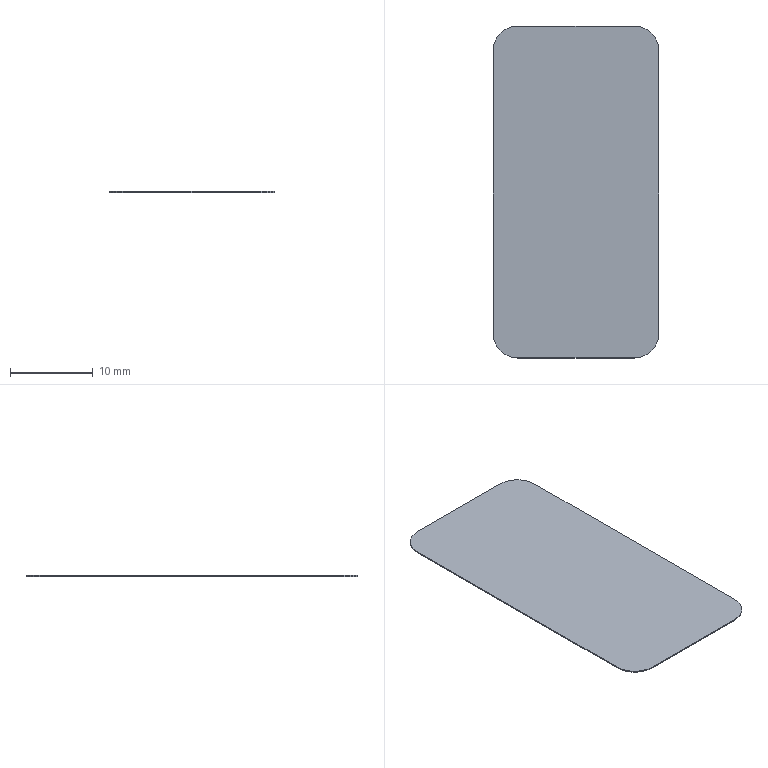Part | STEP file | 68437831 | 1 solid | 10 faces | box 20 x 40 x 0.125 mm | volume 99.034 mm3 | plane 6 | cylinder 4 | commonest cylinder face diameters 6 x4
STEP:
#1=CARTESIAN_POINT('',(0.,0.,0.));
#2=DIRECTION('',(0.,0.,1.));
#3=DIRECTION('',(1.,0.,0.));
#4=AXIS2_PLACEMENT_3D('',#1,#2,#3);
#5=CARTESIAN_POINT('',(7.,20.,0.));
#6=VERTEX_POINT('',#5);
#7=CARTESIAN_POINT('',(10.,17.,0.));
#8=VERTEX_POINT('',#7);
#9=CARTESIAN_POINT('',(7.,17.,0.));
#10=DIRECTION('',(0.,0.,-1.));
#11=DIRECTION('',(0.,1.,0.));
#12=AXIS2_PLACEMENT_3D('',#9,#10,#11);
#13=CIRCLE('',#12,3.);
#14=CARTESIAN_POINT('',(0.,0.,0.));
#15=DIRECTION('',(0.,0.,1.));
#16=DIRECTION('',(1.,0.,0.));
#17=AXIS2_PLACEMENT_3D('',#14,#15,#16);
#18=PLANE('',#17);
#19=CARTESIAN_POINT('',(7.,20.));
#20=CARTESIAN_POINT('',(12.196,20.));
#21=CARTESIAN_POINT('',(9.598,15.5));
#22=CARTESIAN_POINT('',(7.,11.));
#23=CARTESIAN_POINT('',(4.402,15.5));
#24=CARTESIAN_POINT('',(1.804,20.));
#25=CARTESIAN_POINT('',(7.,20.));
#26=(BOUNDED_CURVE()B_SPLINE_CURVE(2,(#19,#20,#21,#22,#23,#24,#25),.UNSPECIFIED.,.T.,.F.)B_SPLINE_CURVE_WITH_KNOTS((1,2,2,2,2,1),(-2.094,0.,2.094,4.189,6.283,8.378),.UNSPECIFIED.)CURVE()GEOMETRIC_REPRESENTATION_ITEM()RATIONAL_B_SPLINE_CURVE((1.,0.5,1.,0.5,1.,0.5,1.))REPRESENTATION_ITEM(''));
#27=(GEOMETRIC_REPRESENTATION_CONTEXT(2)PARAMETRIC_REPRESENTATION_CONTEXT()REPRESENTATION_CONTEXT('',''));
#28=DEFINITIONAL_REPRESENTATION('',(#26),#27);
#29=PCURVE('',#18,#28);
#30=CARTESIAN_POINT('',(7.,17.,0.202));
#31=DIRECTION('',(0.,0.,-1.));
#32=DIRECTION('',(0.,1.,0.));
#33=AXIS2_PLACEMENT_3D('',#30,#31,#32);
#34=CYLINDRICAL_SURFACE('',#33,3.);
#35=CARTESIAN_POINT('',(0.,0.202));
#36=DIRECTION('',(1.,0.));
#37=VECTOR('',#36,1.);
#38=LINE('',#35,#37);
#39=(GEOMETRIC_REPRESENTATION_CONTEXT(2)PARAMETRIC_REPRESENTATION_CONTEXT()REPRESENTATION_CONTEXT('',''));
#40=DEFINITIONAL_REPRESENTATION('',(#38),#39);
#41=PCURVE('',#34,#40);
#42=SURFACE_CURVE('',#13,(#29,#41),.PCURVE_S1.);
#43=EDGE_CURVE('',#6,#8,#42,.T.);
#44=ORIENTED_EDGE('',*,*,#43,.F.);
#45=CARTESIAN_POINT('',(-7.,20.,0.));
#46=VERTEX_POINT('',#45);
#47=CARTESIAN_POINT('',(7.,20.,0.));
#48=DIRECTION('',(-1.,0.,0.));
#49=VECTOR('',#48,1.);
#50=LINE('',#47,#49);
#51=CARTESIAN_POINT('',(7.,20.));
#52=DIRECTION('',(-1.,0.));
#53=VECTOR('',#52,1.);
#54=LINE('',#51,#53);
#55=(GEOMETRIC_REPRESENTATION_CONTEXT(2)PARAMETRIC_REPRESENTATION_CONTEXT()REPRESENTATION_CONTEXT('',''));
#56=DEFINITIONAL_REPRESENTATION('',(#54),#55);
#57=PCURVE('',#18,#56);
#58=CARTESIAN_POINT('',(10.,20.,0.));
#59=DIRECTION('',(0.,1.,0.));
#60=DIRECTION('',(-1.,0.,0.));
#61=AXIS2_PLACEMENT_3D('',#58,#59,#60);
#62=PLANE('',#61);
#63=CARTESIAN_POINT('',(3.,0.));
#64=DIRECTION('',(1.,0.));
#65=VECTOR('',#64,1.);
#66=LINE('',#63,#65);
#67=(GEOMETRIC_REPRESENTATION_CONTEXT(2)PARAMETRIC_REPRESENTATION_CONTEXT()REPRESENTATION_CONTEXT('',''));
#68=DEFINITIONAL_REPRESENTATION('',(#66),#67);
#69=PCURVE('',#62,#68);
#70=SURFACE_CURVE('',#50,(#57,#69),.PCURVE_S1.);
#71=EDGE_CURVE('',#6,#46,#70,.T.);
#72=ORIENTED_EDGE('',*,*,#71,.T.);
#73=CARTESIAN_POINT('',(-10.,17.,0.));
#74=VERTEX_POINT('',#73);
#75=CARTESIAN_POINT('',(-7.,17.,0.));
#76=DIRECTION('',(0.,0.,-1.));
#77=DIRECTION('',(-1.,0.,0.));
#78=AXIS2_PLACEMENT_3D('',#75,#76,#77);
#79=CIRCLE('',#78,3.);
#80=CARTESIAN_POINT('',(-10.,17.));
#81=CARTESIAN_POINT('',(-10.,22.196));
#82=CARTESIAN_POINT('',(-5.5,19.598));
#83=CARTESIAN_POINT('',(-1.,17.));
#84=CARTESIAN_POINT('',(-5.5,14.402));
#85=CARTESIAN_POINT('',(-10.,11.804));
#86=CARTESIAN_POINT('',(-10.,17.));
#87=(BOUNDED_CURVE()B_SPLINE_CURVE(2,(#80,#81,#82,#83,#84,#85,#86),.UNSPECIFIED.,.T.,.F.)B_SPLINE_CURVE_WITH_KNOTS((1,2,2,2,2,1),(-2.094,0.,2.094,4.189,6.283,8.378),.UNSPECIFIED.)CURVE()GEOMETRIC_REPRESENTATION_ITEM()RATIONAL_B_SPLINE_CURVE((1.,0.5,1.,0.5,1.,0.5,1.))REPRESENTATION_ITEM(''));
#88=(GEOMETRIC_REPRESENTATION_CONTEXT(2)PARAMETRIC_REPRESENTATION_CONTEXT()REPRESENTATION_CONTEXT('',''));
#89=DEFINITIONAL_REPRESENTATION('',(#87),#88);
#90=PCURVE('',#18,#89);
#91=CARTESIAN_POINT('',(-7.,17.,0.202));
#92=DIRECTION('',(0.,0.,-1.));
#93=DIRECTION('',(-1.,0.,0.));
#94=AXIS2_PLACEMENT_3D('',#91,#92,#93);
#95=CYLINDRICAL_SURFACE('',#94,3.);
#96=CARTESIAN_POINT('',(0.,0.202));
#97=DIRECTION('',(1.,0.));
#98=VECTOR('',#97,1.);
#99=LINE('',#96,#98);
#100=(GEOMETRIC_REPRESENTATION_CONTEXT(2)PARAMETRIC_REPRESENTATION_CONTEXT()REPRESENTATION_CONTEXT('',''));
#101=DEFINITIONAL_REPRESENTATION('',(#99),#100);
#102=PCURVE('',#95,#101);
#103=SURFACE_CURVE('',#79,(#90,#102),.PCURVE_S1.);
#104=EDGE_CURVE('',#74,#46,#103,.T.);
#105=ORIENTED_EDGE('',*,*,#104,.F.);
#106=CARTESIAN_POINT('',(-10.,-17.,0.));
#107=VERTEX_POINT('',#106);
#108=CARTESIAN_POINT('',(-10.,17.,0.));
#109=DIRECTION('',(0.,-1.,0.));
#110=VECTOR('',#109,1.);
#111=LINE('',#108,#110);
#112=CARTESIAN_POINT('',(-10.,17.));
#113=DIRECTION('',(0.,-1.));
#114=VECTOR('',#113,1.);
#115=LINE('',#112,#114);
#116=(GEOMETRIC_REPRESENTATION_CONTEXT(2)PARAMETRIC_REPRESENTATION_CONTEXT()REPRESENTATION_CONTEXT('',''));
#117=DEFINITIONAL_REPRESENTATION('',(#115),#116);
#118=PCURVE('',#18,#117);
#119=CARTESIAN_POINT('',(-10.,20.,0.));
#120=DIRECTION('',(-1.,0.,0.));
#121=DIRECTION('',(0.,-1.,0.));
#122=AXIS2_PLACEMENT_3D('',#119,#120,#121);
#123=PLANE('',#122);
#124=CARTESIAN_POINT('',(3.,0.));
#125=DIRECTION('',(1.,0.));
#126=VECTOR('',#125,1.);
#127=LINE('',#124,#126);
#128=(GEOMETRIC_REPRESENTATION_CONTEXT(2)PARAMETRIC_REPRESENTATION_CONTEXT()REPRESENTATION_CONTEXT('',''));
#129=DEFINITIONAL_REPRESENTATION('',(#127),#128);
#130=PCURVE('',#123,#129);
#131=SURFACE_CURVE('',#111,(#118,#130),.PCURVE_S1.);
#132=EDGE_CURVE('',#74,#107,#131,.T.);
#133=ORIENTED_EDGE('',*,*,#132,.T.);
#134=CARTESIAN_POINT('',(-7.,-20.,0.));
#135=VERTEX_POINT('',#134);
#136=CARTESIAN_POINT('',(-7.,-17.,0.));
#137=DIRECTION('',(0.,0.,-1.));
#138=DIRECTION('',(0.,-1.,0.));
#139=AXIS2_PLACEMENT_3D('',#136,#137,#138);
#140=CIRCLE('',#139,3.);
#141=CARTESIAN_POINT('',(-7.,-20.));
#142=CARTESIAN_POINT('',(-12.196,-20.));
#143=CARTESIAN_POINT('',(-9.598,-15.5));
#144=CARTESIAN_POINT('',(-7.,-11.));
#145=CARTESIAN_POINT('',(-4.402,-15.5));
#146=CARTESIAN_POINT('',(-1.804,-20.));
#147=CARTESIAN_POINT('',(-7.,-20.));
#148=(BOUNDED_CURVE()B_SPLINE_CURVE(2,(#141,#142,#143,#144,#145,#146,#147),.UNSPECIFIED.,.T.,.F.)B_SPLINE_CURVE_WITH_KNOTS((1,2,2,2,2,1),(-2.094,0.,2.094,4.189,6.283,8.378),.UNSPECIFIED.)CURVE()GEOMETRIC_REPRESENTATION_ITEM()RATIONAL_B_SPLINE_CURVE((1.,0.5,1.,0.5,1.,0.5,1.))REPRESENTATION_ITEM(''));
#149=(GEOMETRIC_REPRESENTATION_CONTEXT(2)PARAMETRIC_REPRESENTATION_CONTEXT()REPRESENTATION_CONTEXT('',''));
#150=DEFINITIONAL_REPRESENTATION('',(#148),#149);
#151=PCURVE('',#18,#150);
#152=CARTESIAN_POINT('',(-7.,-17.,0.202));
#153=DIRECTION('',(0.,0.,-1.));
#154=DIRECTION('',(0.,-1.,0.));
#155=AXIS2_PLACEMENT_3D('',#152,#153,#154);
#156=CYLINDRICAL_SURFACE('',#155,3.);
#157=CARTESIAN_POINT('',(0.,0.202));
#158=DIRECTION('',(1.,0.));
#159=VECTOR('',#158,1.);
#160=LINE('',#157,#159);
#161=(GEOMETRIC_REPRESENTATION_CONTEXT(2)PARAMETRIC_REPRESENTATION_CONTEXT()REPRESENTATION_CONTEXT('',''));
#162=DEFINITIONAL_REPRESENTATION('',(#160),#161);
#163=PCURVE('',#156,#162);
#164=SURFACE_CURVE('',#140,(#151,#163),.PCURVE_S1.);
#165=EDGE_CURVE('',#135,#107,#164,.T.);
#166=ORIENTED_EDGE('',*,*,#165,.F.);
#167=CARTESIAN_POINT('',(7.,-20.,0.));
#168=VERTEX_POINT('',#167);
#169=CARTESIAN_POINT('',(-7.,-20.,0.));
#170=DIRECTION('',(1.,0.,0.));
#171=VECTOR('',#170,1.);
#172=LINE('',#169,#171);
#173=CARTESIAN_POINT('',(-7.,-20.));
#174=DIRECTION('',(1.,0.));
#175=VECTOR('',#174,1.);
#176=LINE('',#173,#175);
#177=(GEOMETRIC_REPRESENTATION_CONTEXT(2)PARAMETRIC_REPRESENTATION_CONTEXT()REPRESENTATION_CONTEXT('',''));
#178=DEFINITIONAL_REPRESENTATION('',(#176),#177);
#179=PCURVE('',#18,#178);
#180=CARTESIAN_POINT('',(-10.,-20.,0.));
#181=DIRECTION('',(0.,-1.,0.));
#182=DIRECTION('',(1.,0.,0.));
#183=AXIS2_PLACEMENT_3D('',#180,#181,#182);
#184=PLANE('',#183);
#185=CARTESIAN_POINT('',(3.,0.));
#186=DIRECTION('',(1.,0.));
#187=VECTOR('',#186,1.);
#188=LINE('',#185,#187);
#189=(GEOMETRIC_REPRESENTATION_CONTEXT(2)PARAMETRIC_REPRESENTATION_CONTEXT()REPRESENTATION_CONTEXT('',''));
#190=DEFINITIONAL_REPRESENTATION('',(#188),#189);
#191=PCURVE('',#184,#190);
#192=SURFACE_CURVE('',#172,(#179,#191),.PCURVE_S1.);
#193=EDGE_CURVE('',#135,#168,#192,.T.);
#194=ORIENTED_EDGE('',*,*,#193,.T.);
#195=CARTESIAN_POINT('',(10.,-17.,0.));
#196=VERTEX_POINT('',#195);
#197=CARTESIAN_POINT('',(7.,-17.,0.));
#198=DIRECTION('',(0.,0.,-1.));
#199=DIRECTION('',(1.,0.,0.));
#200=AXIS2_PLACEMENT_3D('',#197,#198,#199);
#201=CIRCLE('',#200,3.);
#202=CARTESIAN_POINT('',(10.,-17.));
#203=CARTESIAN_POINT('',(10.,-22.196));
#204=CARTESIAN_POINT('',(5.5,-19.598));
#205=CARTESIAN_POINT('',(1.,-17.));
#206=CARTESIAN_POINT('',(5.5,-14.402));
#207=CARTESIAN_POINT('',(10.,-11.804));
#208=CARTESIAN_POINT('',(10.,-17.));
#209=(BOUNDED_CURVE()B_SPLINE_CURVE(2,(#202,#203,#204,#205,#206,#207,#208),.UNSPECIFIED.,.T.,.F.)B_SPLINE_CURVE_WITH_KNOTS((1,2,2,2,2,1),(-2.094,0.,2.094,4.189,6.283,8.378),.UNSPECIFIED.)CURVE()GEOMETRIC_REPRESENTATION_ITEM()RATIONAL_B_SPLINE_CURVE((1.,0.5,1.,0.5,1.,0.5,1.))REPRESENTATION_ITEM(''));
#210=(GEOMETRIC_REPRESENTATION_CONTEXT(2)PARAMETRIC_REPRESENTATION_CONTEXT()REPRESENTATION_CONTEXT('',''));
#211=DEFINITIONAL_REPRESENTATION('',(#209),#210);
#212=PCURVE('',#18,#211);
#213=CARTESIAN_POINT('',(7.,-17.,0.202));
#214=DIRECTION('',(0.,0.,-1.));
#215=DIRECTION('',(1.,0.,0.));
#216=AXIS2_PLACEMENT_3D('',#213,#214,#215);
#217=CYLINDRICAL_SURFACE('',#216,3.);
#218=CARTESIAN_POINT('',(0.,0.202));
#219=DIRECTION('',(1.,0.));
#220=VECTOR('',#219,1.);
#221=LINE('',#218,#220);
#222=(GEOMETRIC_REPRESENTATION_CONTEXT(2)PARAMETRIC_REPRESENTATION_CONTEXT()REPRESENTATION_CONTEXT('',''));
#223=DEFINITIONAL_REPRESENTATION('',(#221),#222);
#224=PCURVE('',#217,#223);
#225=SURFACE_CURVE('',#201,(#212,#224),.PCURVE_S1.);
#226=EDGE_CURVE('',#196,#168,#225,.T.);
#227=ORIENTED_EDGE('',*,*,#226,.F.);
#228=CARTESIAN_POINT('',(10.,-17.,0.));
#229=DIRECTION('',(0.,1.,0.));
#230=VECTOR('',#229,1.);
#231=LINE('',#228,#230);
#232=CARTESIAN_POINT('',(10.,-17.));
#233=DIRECTION('',(0.,1.));
#234=VECTOR('',#233,1.);
#235=LINE('',#232,#234);
#236=(GEOMETRIC_REPRESENTATION_CONTEXT(2)PARAMETRIC_REPRESENTATION_CONTEXT()REPRESENTATION_CONTEXT('',''));
#237=DEFINITIONAL_REPRESENTATION('',(#235),#236);
#238=PCURVE('',#18,#237);
#239=CARTESIAN_POINT('',(10.,-20.,0.));
#240=DIRECTION('',(1.,0.,0.));
#241=DIRECTION('',(0.,1.,0.));
#242=AXIS2_PLACEMENT_3D('',#239,#240,#241);
#243=PLANE('',#242);
#244=CARTESIAN_POINT('',(3.,0.));
#245=DIRECTION('',(1.,0.));
#246=VECTOR('',#245,1.);
#247=LINE('',#244,#246);
#248=(GEOMETRIC_REPRESENTATION_CONTEXT(2)PARAMETRIC_REPRESENTATION_CONTEXT()REPRESENTATION_CONTEXT('',''));
#249=DEFINITIONAL_REPRESENTATION('',(#247),#248);
#250=PCURVE('',#243,#249);
#251=SURFACE_CURVE('',#231,(#238,#250),.PCURVE_S1.);
#252=EDGE_CURVE('',#196,#8,#251,.T.);
#253=ORIENTED_EDGE('',*,*,#252,.T.);
#254=EDGE_LOOP('',(#44,#72,#105,#133,#166,#194,#227,#253));
#255=FACE_BOUND('',#254,.F.);
#256=ADVANCED_FACE('',(#255),#18,.F.);
#257=ORIENTED_EDGE('',*,*,#43,.F.);
#258=CARTESIAN_POINT('',(7.,20.,0.125));
#259=VERTEX_POINT('',#258);
#260=CARTESIAN_POINT('',(7.,20.,0.125));
#261=DIRECTION('',(0.,0.,-1.));
#262=VECTOR('',#261,1.);
#263=LINE('',#260,#262);
#264=CARTESIAN_POINT('',(0.,0.07697));
#265=DIRECTION('',(0.,1.));
#266=VECTOR('',#265,1.);
#267=LINE('',#264,#266);
#268=(GEOMETRIC_REPRESENTATION_CONTEXT(2)PARAMETRIC_REPRESENTATION_CONTEXT()REPRESENTATION_CONTEXT('',''));
#269=DEFINITIONAL_REPRESENTATION('',(#267),#268);
#270=PCURVE('',#34,#269);
#271=CARTESIAN_POINT('',(3.,0.125));
#272=DIRECTION('',(0.,-1.));
#273=VECTOR('',#272,1.);
#274=LINE('',#271,#273);
#275=(GEOMETRIC_REPRESENTATION_CONTEXT(2)PARAMETRIC_REPRESENTATION_CONTEXT()REPRESENTATION_CONTEXT('',''));
#276=DEFINITIONAL_REPRESENTATION('',(#274),#275);
#277=PCURVE('',#62,#276);
#278=SURFACE_CURVE('',#263,(#270,#277),.PCURVE_S1.);
#279=EDGE_CURVE('',#259,#6,#278,.T.);
#280=ORIENTED_EDGE('',*,*,#279,.F.);
#281=CARTESIAN_POINT('',(10.,17.,0.125));
#282=VERTEX_POINT('',#281);
#283=CARTESIAN_POINT('',(7.,17.,0.125));
#284=DIRECTION('',(0.,0.,1.));
#285=DIRECTION('',(1.,0.,0.));
#286=AXIS2_PLACEMENT_3D('',#283,#284,#285);
#287=CIRCLE('',#286,3.);
#288=CARTESIAN_POINT('',(1.571,0.07697));
#289=DIRECTION('',(-1.,0.));
#290=VECTOR('',#289,1.);
#291=LINE('',#288,#290);
#292=(GEOMETRIC_REPRESENTATION_CONTEXT(2)PARAMETRIC_REPRESENTATION_CONTEXT()REPRESENTATION_CONTEXT('',''));
#293=DEFINITIONAL_REPRESENTATION('',(#291),#292);
#294=PCURVE('',#34,#293);
#295=CARTESIAN_POINT('',(0.,0.,0.125));
#296=DIRECTION('',(0.,0.,1.));
#297=DIRECTION('',(1.,0.,0.));
#298=AXIS2_PLACEMENT_3D('',#295,#296,#297);
#299=PLANE('',#298);
#300=CARTESIAN_POINT('',(7.,17.));
#301=DIRECTION('',(1.,0.));
#302=AXIS2_PLACEMENT_2D('',#300,#301);
#303=CIRCLE('',#302,3.);
#304=(GEOMETRIC_REPRESENTATION_CONTEXT(2)PARAMETRIC_REPRESENTATION_CONTEXT()REPRESENTATION_CONTEXT('',''));
#305=DEFINITIONAL_REPRESENTATION('',(#303),#304);
#306=PCURVE('',#299,#305);
#307=SURFACE_CURVE('',#287,(#294,#306),.PCURVE_S1.);
#308=EDGE_CURVE('',#282,#259,#307,.T.);
#309=ORIENTED_EDGE('',*,*,#308,.F.);
#310=CARTESIAN_POINT('',(10.,17.,0.125));
#311=DIRECTION('',(0.,0.,-1.));
#312=VECTOR('',#311,1.);
#313=LINE('',#310,#312);
#314=CARTESIAN_POINT('',(1.571,0.07697));
#315=DIRECTION('',(0.,1.));
#316=VECTOR('',#315,1.);
#317=LINE('',#314,#316);
#318=(GEOMETRIC_REPRESENTATION_CONTEXT(2)PARAMETRIC_REPRESENTATION_CONTEXT()REPRESENTATION_CONTEXT('',''));
#319=DEFINITIONAL_REPRESENTATION('',(#317),#318);
#320=PCURVE('',#34,#319);
#321=CARTESIAN_POINT('',(37.,0.125));
#322=DIRECTION('',(0.,-1.));
#323=VECTOR('',#322,1.);
#324=LINE('',#321,#323);
#325=(GEOMETRIC_REPRESENTATION_CONTEXT(2)PARAMETRIC_REPRESENTATION_CONTEXT()REPRESENTATION_CONTEXT('',''));
#326=DEFINITIONAL_REPRESENTATION('',(#324),#325);
#327=PCURVE('',#243,#326);
#328=SURFACE_CURVE('',#313,(#320,#327),.PCURVE_S1.);
#329=EDGE_CURVE('',#282,#8,#328,.T.);
#330=ORIENTED_EDGE('',*,*,#329,.T.);
#331=EDGE_LOOP('',(#257,#280,#309,#330));
#332=FACE_BOUND('',#331,.T.);
#333=ADVANCED_FACE('',(#332),#34,.T.);
#334=ORIENTED_EDGE('',*,*,#329,.T.);
#335=ORIENTED_EDGE('',*,*,#252,.F.);
#336=CARTESIAN_POINT('',(10.,-17.,0.125));
#337=VERTEX_POINT('',#336);
#338=CARTESIAN_POINT('',(10.,-17.,0.125));
#339=DIRECTION('',(0.,0.,-1.));
#340=VECTOR('',#339,1.);
#341=LINE('',#338,#340);
#342=CARTESIAN_POINT('',(3.,0.125));
#343=DIRECTION('',(0.,-1.));
#344=VECTOR('',#343,1.);
#345=LINE('',#342,#344);
#346=(GEOMETRIC_REPRESENTATION_CONTEXT(2)PARAMETRIC_REPRESENTATION_CONTEXT()REPRESENTATION_CONTEXT('',''));
#347=DEFINITIONAL_REPRESENTATION('',(#345),#346);
#348=PCURVE('',#243,#347);
#349=CARTESIAN_POINT('',(0.,0.07697));
#350=DIRECTION('',(0.,1.));
#351=VECTOR('',#350,1.);
#352=LINE('',#349,#351);
#353=(GEOMETRIC_REPRESENTATION_CONTEXT(2)PARAMETRIC_REPRESENTATION_CONTEXT()REPRESENTATION_CONTEXT('',''));
#354=DEFINITIONAL_REPRESENTATION('',(#352),#353);
#355=PCURVE('',#217,#354);
#356=SURFACE_CURVE('',#341,(#348,#355),.PCURVE_S1.);
#357=EDGE_CURVE('',#337,#196,#356,.T.);
#358=ORIENTED_EDGE('',*,*,#357,.F.);
#359=CARTESIAN_POINT('',(10.,-17.,0.125));
#360=DIRECTION('',(0.,1.,0.));
#361=VECTOR('',#360,1.);
#362=LINE('',#359,#361);
#363=CARTESIAN_POINT('',(3.,0.125));
#364=DIRECTION('',(1.,0.));
#365=VECTOR('',#364,1.);
#366=LINE('',#363,#365);
#367=(GEOMETRIC_REPRESENTATION_CONTEXT(2)PARAMETRIC_REPRESENTATION_CONTEXT()REPRESENTATION_CONTEXT('',''));
#368=DEFINITIONAL_REPRESENTATION('',(#366),#367);
#369=PCURVE('',#243,#368);
#370=CARTESIAN_POINT('',(10.,-17.));
#371=DIRECTION('',(0.,1.));
#372=VECTOR('',#371,1.);
#373=LINE('',#370,#372);
#374=(GEOMETRIC_REPRESENTATION_CONTEXT(2)PARAMETRIC_REPRESENTATION_CONTEXT()REPRESENTATION_CONTEXT('',''));
#375=DEFINITIONAL_REPRESENTATION('',(#373),#374);
#376=PCURVE('',#299,#375);
#377=SURFACE_CURVE('',#362,(#369,#376),.PCURVE_S1.);
#378=EDGE_CURVE('',#337,#282,#377,.T.);
#379=ORIENTED_EDGE('',*,*,#378,.T.);
#380=EDGE_LOOP('',(#334,#335,#358,#379));
#381=FACE_BOUND('',#380,.F.);
#382=ADVANCED_FACE('',(#381),#243,.T.);
#383=ORIENTED_EDGE('',*,*,#226,.F.);
#384=ORIENTED_EDGE('',*,*,#357,.F.);
#385=CARTESIAN_POINT('',(7.,-20.,0.125));
#386=VERTEX_POINT('',#385);
#387=CARTESIAN_POINT('',(7.,-17.,0.125));
#388=DIRECTION('',(0.,0.,1.));
#389=DIRECTION('',(0.,-1.,0.));
#390=AXIS2_PLACEMENT_3D('',#387,#388,#389);
#391=CIRCLE('',#390,3.);
#392=CARTESIAN_POINT('',(1.571,0.07697));
#393=DIRECTION('',(-1.,0.));
#394=VECTOR('',#393,1.);
#395=LINE('',#392,#394);
#396=(GEOMETRIC_REPRESENTATION_CONTEXT(2)PARAMETRIC_REPRESENTATION_CONTEXT()REPRESENTATION_CONTEXT('',''));
#397=DEFINITIONAL_REPRESENTATION('',(#395),#396);
#398=PCURVE('',#217,#397);
#399=CARTESIAN_POINT('',(7.,-17.));
#400=DIRECTION('',(0.,-1.));
#401=AXIS2_PLACEMENT_2D('',#399,#400);
#402=CIRCLE('',#401,3.);
#403=(GEOMETRIC_REPRESENTATION_CONTEXT(2)PARAMETRIC_REPRESENTATION_CONTEXT()REPRESENTATION_CONTEXT('',''));
#404=DEFINITIONAL_REPRESENTATION('',(#402),#403);
#405=PCURVE('',#299,#404);
#406=SURFACE_CURVE('',#391,(#398,#405),.PCURVE_S1.);
#407=EDGE_CURVE('',#386,#337,#406,.T.);
#408=ORIENTED_EDGE('',*,*,#407,.F.);
#409=CARTESIAN_POINT('',(7.,-20.,0.125));
#410=DIRECTION('',(0.,0.,-1.));
#411=VECTOR('',#410,1.);
#412=LINE('',#409,#411);
#413=CARTESIAN_POINT('',(1.571,0.07697));
#414=DIRECTION('',(0.,1.));
#415=VECTOR('',#414,1.);
#416=LINE('',#413,#415);
#417=(GEOMETRIC_REPRESENTATION_CONTEXT(2)PARAMETRIC_REPRESENTATION_CONTEXT()REPRESENTATION_CONTEXT('',''));
#418=DEFINITIONAL_REPRESENTATION('',(#416),#417);
#419=PCURVE('',#217,#418);
#420=CARTESIAN_POINT('',(17.,0.125));
#421=DIRECTION('',(0.,-1.));
#422=VECTOR('',#421,1.);
#423=LINE('',#420,#422);
#424=(GEOMETRIC_REPRESENTATION_CONTEXT(2)PARAMETRIC_REPRESENTATION_CONTEXT()REPRESENTATION_CONTEXT('',''));
#425=DEFINITIONAL_REPRESENTATION('',(#423),#424);
#426=PCURVE('',#184,#425);
#427=SURFACE_CURVE('',#412,(#419,#426),.PCURVE_S1.);
#428=EDGE_CURVE('',#386,#168,#427,.T.);
#429=ORIENTED_EDGE('',*,*,#428,.T.);
#430=EDGE_LOOP('',(#383,#384,#408,#429));
#431=FACE_BOUND('',#430,.T.);
#432=ADVANCED_FACE('',(#431),#217,.T.);
#433=ORIENTED_EDGE('',*,*,#428,.T.);
#434=ORIENTED_EDGE('',*,*,#193,.F.);
#435=CARTESIAN_POINT('',(-7.,-20.,0.125));
#436=VERTEX_POINT('',#435);
#437=CARTESIAN_POINT('',(-7.,-20.,0.125));
#438=DIRECTION('',(0.,0.,-1.));
#439=VECTOR('',#438,1.);
#440=LINE('',#437,#439);
#441=CARTESIAN_POINT('',(3.,0.125));
#442=DIRECTION('',(0.,-1.));
#443=VECTOR('',#442,1.);
#444=LINE('',#441,#443);
#445=(GEOMETRIC_REPRESENTATION_CONTEXT(2)PARAMETRIC_REPRESENTATION_CONTEXT()REPRESENTATION_CONTEXT('',''));
#446=DEFINITIONAL_REPRESENTATION('',(#444),#445);
#447=PCURVE('',#184,#446);
#448=CARTESIAN_POINT('',(0.,0.07697));
#449=DIRECTION('',(0.,1.));
#450=VECTOR('',#449,1.);
#451=LINE('',#448,#450);
#452=(GEOMETRIC_REPRESENTATION_CONTEXT(2)PARAMETRIC_REPRESENTATION_CONTEXT()REPRESENTATION_CONTEXT('',''));
#453=DEFINITIONAL_REPRESENTATION('',(#451),#452);
#454=PCURVE('',#156,#453);
#455=SURFACE_CURVE('',#440,(#447,#454),.PCURVE_S1.);
#456=EDGE_CURVE('',#436,#135,#455,.T.);
#457=ORIENTED_EDGE('',*,*,#456,.F.);
#458=CARTESIAN_POINT('',(-7.,-20.,0.125));
#459=DIRECTION('',(1.,0.,0.));
#460=VECTOR('',#459,1.);
#461=LINE('',#458,#460);
#462=CARTESIAN_POINT('',(3.,0.125));
#463=DIRECTION('',(1.,0.));
#464=VECTOR('',#463,1.);
#465=LINE('',#462,#464);
#466=(GEOMETRIC_REPRESENTATION_CONTEXT(2)PARAMETRIC_REPRESENTATION_CONTEXT()REPRESENTATION_CONTEXT('',''));
#467=DEFINITIONAL_REPRESENTATION('',(#465),#466);
#468=PCURVE('',#184,#467);
#469=CARTESIAN_POINT('',(-7.,-20.));
#470=DIRECTION('',(1.,0.));
#471=VECTOR('',#470,1.);
#472=LINE('',#469,#471);
#473=(GEOMETRIC_REPRESENTATION_CONTEXT(2)PARAMETRIC_REPRESENTATION_CONTEXT()REPRESENTATION_CONTEXT('',''));
#474=DEFINITIONAL_REPRESENTATION('',(#472),#473);
#475=PCURVE('',#299,#474);
#476=SURFACE_CURVE('',#461,(#468,#475),.PCURVE_S1.);
#477=EDGE_CURVE('',#436,#386,#476,.T.);
#478=ORIENTED_EDGE('',*,*,#477,.T.);
#479=EDGE_LOOP('',(#433,#434,#457,#478));
#480=FACE_BOUND('',#479,.F.);
#481=ADVANCED_FACE('',(#480),#184,.T.);
#482=ORIENTED_EDGE('',*,*,#165,.F.);
#483=ORIENTED_EDGE('',*,*,#456,.F.);
#484=CARTESIAN_POINT('',(-10.,-17.,0.125));
#485=VERTEX_POINT('',#484);
#486=CARTESIAN_POINT('',(-7.,-17.,0.125));
#487=DIRECTION('',(0.,0.,1.));
#488=DIRECTION('',(-1.,0.,0.));
#489=AXIS2_PLACEMENT_3D('',#486,#487,#488);
#490=CIRCLE('',#489,3.);
#491=CARTESIAN_POINT('',(1.571,0.07697));
#492=DIRECTION('',(-1.,0.));
#493=VECTOR('',#492,1.);
#494=LINE('',#491,#493);
#495=(GEOMETRIC_REPRESENTATION_CONTEXT(2)PARAMETRIC_REPRESENTATION_CONTEXT()REPRESENTATION_CONTEXT('',''));
#496=DEFINITIONAL_REPRESENTATION('',(#494),#495);
#497=PCURVE('',#156,#496);
#498=CARTESIAN_POINT('',(-7.,-17.));
#499=DIRECTION('',(-1.,0.));
#500=AXIS2_PLACEMENT_2D('',#498,#499);
#501=CIRCLE('',#500,3.);
#502=(GEOMETRIC_REPRESENTATION_CONTEXT(2)PARAMETRIC_REPRESENTATION_CONTEXT()REPRESENTATION_CONTEXT('',''));
#503=DEFINITIONAL_REPRESENTATION('',(#501),#502);
#504=PCURVE('',#299,#503);
#505=SURFACE_CURVE('',#490,(#497,#504),.PCURVE_S1.);
#506=EDGE_CURVE('',#485,#436,#505,.T.);
#507=ORIENTED_EDGE('',*,*,#506,.F.);
#508=CARTESIAN_POINT('',(-10.,-17.,0.125));
#509=DIRECTION('',(0.,0.,-1.));
#510=VECTOR('',#509,1.);
#511=LINE('',#508,#510);
#512=CARTESIAN_POINT('',(1.571,0.07697));
#513=DIRECTION('',(0.,1.));
#514=VECTOR('',#513,1.);
#515=LINE('',#512,#514);
#516=(GEOMETRIC_REPRESENTATION_CONTEXT(2)PARAMETRIC_REPRESENTATION_CONTEXT()REPRESENTATION_CONTEXT('',''));
#517=DEFINITIONAL_REPRESENTATION('',(#515),#516);
#518=PCURVE('',#156,#517);
#519=CARTESIAN_POINT('',(37.,0.125));
#520=DIRECTION('',(0.,-1.));
#521=VECTOR('',#520,1.);
#522=LINE('',#519,#521);
#523=(GEOMETRIC_REPRESENTATION_CONTEXT(2)PARAMETRIC_REPRESENTATION_CONTEXT()REPRESENTATION_CONTEXT('',''));
#524=DEFINITIONAL_REPRESENTATION('',(#522),#523);
#525=PCURVE('',#123,#524);
#526=SURFACE_CURVE('',#511,(#518,#525),.PCURVE_S1.);
#527=EDGE_CURVE('',#485,#107,#526,.T.);
#528=ORIENTED_EDGE('',*,*,#527,.T.);
#529=EDGE_LOOP('',(#482,#483,#507,#528));
#530=FACE_BOUND('',#529,.T.);
#531=ADVANCED_FACE('',(#530),#156,.T.);
#532=ORIENTED_EDGE('',*,*,#527,.T.);
#533=ORIENTED_EDGE('',*,*,#132,.F.);
#534=CARTESIAN_POINT('',(-10.,17.,0.125));
#535=VERTEX_POINT('',#534);
#536=CARTESIAN_POINT('',(-10.,17.,0.125));
#537=DIRECTION('',(0.,0.,-1.));
#538=VECTOR('',#537,1.);
#539=LINE('',#536,#538);
#540=CARTESIAN_POINT('',(3.,0.125));
#541=DIRECTION('',(0.,-1.));
#542=VECTOR('',#541,1.);
#543=LINE('',#540,#542);
#544=(GEOMETRIC_REPRESENTATION_CONTEXT(2)PARAMETRIC_REPRESENTATION_CONTEXT()REPRESENTATION_CONTEXT('',''));
#545=DEFINITIONAL_REPRESENTATION('',(#543),#544);
#546=PCURVE('',#123,#545);
#547=CARTESIAN_POINT('',(0.,0.07697));
#548=DIRECTION('',(0.,1.));
#549=VECTOR('',#548,1.);
#550=LINE('',#547,#549);
#551=(GEOMETRIC_REPRESENTATION_CONTEXT(2)PARAMETRIC_REPRESENTATION_CONTEXT()REPRESENTATION_CONTEXT('',''));
#552=DEFINITIONAL_REPRESENTATION('',(#550),#551);
#553=PCURVE('',#95,#552);
#554=SURFACE_CURVE('',#539,(#546,#553),.PCURVE_S1.);
#555=EDGE_CURVE('',#535,#74,#554,.T.);
#556=ORIENTED_EDGE('',*,*,#555,.F.);
#557=CARTESIAN_POINT('',(-10.,17.,0.125));
#558=DIRECTION('',(0.,-1.,0.));
#559=VECTOR('',#558,1.);
#560=LINE('',#557,#559);
#561=CARTESIAN_POINT('',(3.,0.125));
#562=DIRECTION('',(1.,0.));
#563=VECTOR('',#562,1.);
#564=LINE('',#561,#563);
#565=(GEOMETRIC_REPRESENTATION_CONTEXT(2)PARAMETRIC_REPRESENTATION_CONTEXT()REPRESENTATION_CONTEXT('',''));
#566=DEFINITIONAL_REPRESENTATION('',(#564),#565);
#567=PCURVE('',#123,#566);
#568=CARTESIAN_POINT('',(-10.,17.));
#569=DIRECTION('',(0.,-1.));
#570=VECTOR('',#569,1.);
#571=LINE('',#568,#570);
#572=(GEOMETRIC_REPRESENTATION_CONTEXT(2)PARAMETRIC_REPRESENTATION_CONTEXT()REPRESENTATION_CONTEXT('',''));
#573=DEFINITIONAL_REPRESENTATION('',(#571),#572);
#574=PCURVE('',#299,#573);
#575=SURFACE_CURVE('',#560,(#567,#574),.PCURVE_S1.);
#576=EDGE_CURVE('',#535,#485,#575,.T.);
#577=ORIENTED_EDGE('',*,*,#576,.T.);
#578=EDGE_LOOP('',(#532,#533,#556,#577));
#579=FACE_BOUND('',#578,.F.);
#580=ADVANCED_FACE('',(#579),#123,.T.);
#581=ORIENTED_EDGE('',*,*,#104,.F.);
#582=ORIENTED_EDGE('',*,*,#555,.F.);
#583=CARTESIAN_POINT('',(-7.,20.,0.125));
#584=VERTEX_POINT('',#583);
#585=CARTESIAN_POINT('',(-7.,17.,0.125));
#586=DIRECTION('',(0.,0.,1.));
#587=DIRECTION('',(0.,1.,0.));
#588=AXIS2_PLACEMENT_3D('',#585,#586,#587);
#589=CIRCLE('',#588,3.);
#590=CARTESIAN_POINT('',(1.571,0.07697));
#591=DIRECTION('',(-1.,0.));
#592=VECTOR('',#591,1.);
#593=LINE('',#590,#592);
#594=(GEOMETRIC_REPRESENTATION_CONTEXT(2)PARAMETRIC_REPRESENTATION_CONTEXT()REPRESENTATION_CONTEXT('',''));
#595=DEFINITIONAL_REPRESENTATION('',(#593),#594);
#596=PCURVE('',#95,#595);
#597=CARTESIAN_POINT('',(-7.,17.));
#598=DIRECTION('',(0.,1.));
#599=AXIS2_PLACEMENT_2D('',#597,#598);
#600=CIRCLE('',#599,3.);
#601=(GEOMETRIC_REPRESENTATION_CONTEXT(2)PARAMETRIC_REPRESENTATION_CONTEXT()REPRESENTATION_CONTEXT('',''));
#602=DEFINITIONAL_REPRESENTATION('',(#600),#601);
#603=PCURVE('',#299,#602);
#604=SURFACE_CURVE('',#589,(#596,#603),.PCURVE_S1.);
#605=EDGE_CURVE('',#584,#535,#604,.T.);
#606=ORIENTED_EDGE('',*,*,#605,.F.);
#607=CARTESIAN_POINT('',(-7.,20.,0.125));
#608=DIRECTION('',(0.,0.,-1.));
#609=VECTOR('',#608,1.);
#610=LINE('',#607,#609);
#611=CARTESIAN_POINT('',(1.571,0.07697));
#612=DIRECTION('',(0.,1.));
#613=VECTOR('',#612,1.);
#614=LINE('',#611,#613);
#615=(GEOMETRIC_REPRESENTATION_CONTEXT(2)PARAMETRIC_REPRESENTATION_CONTEXT()REPRESENTATION_CONTEXT('',''));
#616=DEFINITIONAL_REPRESENTATION('',(#614),#615);
#617=PCURVE('',#95,#616);
#618=CARTESIAN_POINT('',(17.,0.125));
#619=DIRECTION('',(0.,-1.));
#620=VECTOR('',#619,1.);
#621=LINE('',#618,#620);
#622=(GEOMETRIC_REPRESENTATION_CONTEXT(2)PARAMETRIC_REPRESENTATION_CONTEXT()REPRESENTATION_CONTEXT('',''));
#623=DEFINITIONAL_REPRESENTATION('',(#621),#622);
#624=PCURVE('',#62,#623);
#625=SURFACE_CURVE('',#610,(#617,#624),.PCURVE_S1.);
#626=EDGE_CURVE('',#584,#46,#625,.T.);
#627=ORIENTED_EDGE('',*,*,#626,.T.);
#628=EDGE_LOOP('',(#581,#582,#606,#627));
#629=FACE_BOUND('',#628,.T.);
#630=ADVANCED_FACE('',(#629),#95,.T.);
#631=ORIENTED_EDGE('',*,*,#279,.F.);
#632=CARTESIAN_POINT('',(7.,20.,0.125));
#633=DIRECTION('',(-1.,0.,0.));
#634=VECTOR('',#633,1.);
#635=LINE('',#632,#634);
#636=CARTESIAN_POINT('',(3.,0.125));
#637=DIRECTION('',(1.,0.));
#638=VECTOR('',#637,1.);
#639=LINE('',#636,#638);
#640=(GEOMETRIC_REPRESENTATION_CONTEXT(2)PARAMETRIC_REPRESENTATION_CONTEXT()REPRESENTATION_CONTEXT('',''));
#641=DEFINITIONAL_REPRESENTATION('',(#639),#640);
#642=PCURVE('',#62,#641);
#643=CARTESIAN_POINT('',(7.,20.));
#644=DIRECTION('',(-1.,0.));
#645=VECTOR('',#644,1.);
#646=LINE('',#643,#645);
#647=(GEOMETRIC_REPRESENTATION_CONTEXT(2)PARAMETRIC_REPRESENTATION_CONTEXT()REPRESENTATION_CONTEXT('',''));
#648=DEFINITIONAL_REPRESENTATION('',(#646),#647);
#649=PCURVE('',#299,#648);
#650=SURFACE_CURVE('',#635,(#642,#649),.PCURVE_S1.);
#651=EDGE_CURVE('',#259,#584,#650,.T.);
#652=ORIENTED_EDGE('',*,*,#651,.T.);
#653=ORIENTED_EDGE('',*,*,#626,.T.);
#654=ORIENTED_EDGE('',*,*,#71,.F.);
#655=EDGE_LOOP('',(#631,#652,#653,#654));
#656=FACE_BOUND('',#655,.F.);
#657=ADVANCED_FACE('',(#656),#62,.T.);
#658=ORIENTED_EDGE('',*,*,#308,.F.);
#659=ORIENTED_EDGE('',*,*,#378,.F.);
#660=ORIENTED_EDGE('',*,*,#407,.F.);
#661=ORIENTED_EDGE('',*,*,#477,.F.);
#662=ORIENTED_EDGE('',*,*,#506,.F.);
#663=ORIENTED_EDGE('',*,*,#576,.F.);
#664=ORIENTED_EDGE('',*,*,#605,.F.);
#665=ORIENTED_EDGE('',*,*,#651,.F.);
#666=EDGE_LOOP('',(#658,#659,#660,#661,#662,#663,#664,#665));
#667=FACE_BOUND('',#666,.F.);
#668=ADVANCED_FACE('',(#667),#299,.T.);
#669=CLOSED_SHELL('',(#256,#333,#382,#432,#481,#531,#580,#630,#657,#668));
#670=MANIFOLD_SOLID_BREP('',#669);
#671=(LENGTH_UNIT()NAMED_UNIT(*)SI_UNIT(.MILLI.,.METRE.));
#672=UNCERTAINTY_MEASURE_WITH_UNIT(LENGTH_MEASURE(0.0000001),#671,'','');
#673=(NAMED_UNIT(*)PLANE_ANGLE_UNIT()SI_UNIT($,.RADIAN.));
#674=(NAMED_UNIT(*)SI_UNIT($,.STERADIAN.)SOLID_ANGLE_UNIT());
#675=(GEOMETRIC_REPRESENTATION_CONTEXT(3)GLOBAL_UNCERTAINTY_ASSIGNED_CONTEXT((#672))GLOBAL_UNIT_ASSIGNED_CONTEXT((#671,#673,#674))REPRESENTATION_CONTEXT('',''));
#676=ADVANCED_BREP_SHAPE_REPRESENTATION('',(#4,#670),#675);